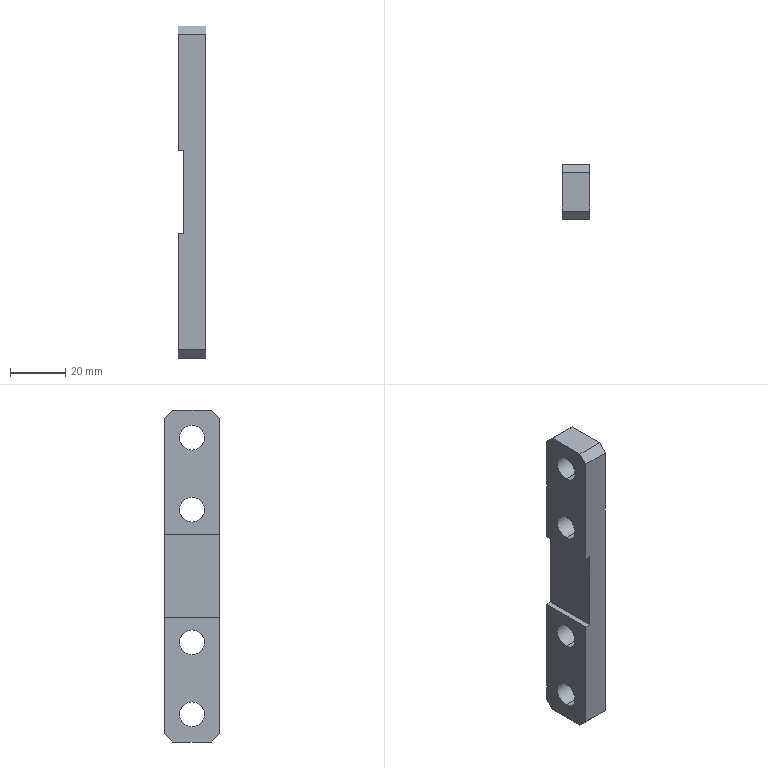Part | SolidWorks | features HoleWzd 2, Chamfer 1, Extrusion 1, ICE 1 | 1 solid | 22 faces | box 10 x 20 x 120 mm | volume 20075 mm3 | plane 14 | cylinder 8 | commonest cylinder face diameters 9 x8
STEP:
#1=CARTESIAN_POINT('',(10.,0.,-54.5));
#2=VERTEX_POINT('',#1);
#3=CARTESIAN_POINT('',(10.,0.,-45.5));
#4=VERTEX_POINT('',#3);
#5=CARTESIAN_POINT('',(10.,0.,-50.));
#6=DIRECTION('',(-1.,0.,0.));
#7=DIRECTION('',(0.,0.,1.));
#8=AXIS2_PLACEMENT_3D('',#5,#6,#7);
#9=CIRCLE('',#8,4.5);
#10=EDGE_CURVE('',#2,#4,#9,.T.);
#11=ORIENTED_EDGE('',*,*,#10,.F.);
#12=CARTESIAN_POINT('',(0.,0.,-54.5));
#13=VERTEX_POINT('',#12);
#14=CARTESIAN_POINT('',(0.,0.,-54.5));
#15=DIRECTION('',(-1.,0.,0.));
#16=VECTOR('',#15,1000.);
#17=LINE('',#14,#16);
#18=EDGE_CURVE('',#2,#13,#17,.T.);
#19=ORIENTED_EDGE('',*,*,#18,.T.);
#20=CARTESIAN_POINT('',(0.,0.,-45.5));
#21=VERTEX_POINT('',#20);
#22=CARTESIAN_POINT('',(0.,0.,-50.));
#23=DIRECTION('',(-1.,0.,0.));
#24=DIRECTION('',(0.,0.,1.));
#25=AXIS2_PLACEMENT_3D('',#22,#23,#24);
#26=CIRCLE('',#25,4.5);
#27=EDGE_CURVE('',#13,#21,#26,.T.);
#28=ORIENTED_EDGE('',*,*,#27,.T.);
#29=CARTESIAN_POINT('',(0.,0.,-45.5));
#30=DIRECTION('',(-1.,0.,0.));
#31=VECTOR('',#30,1000.);
#32=LINE('',#29,#31);
#33=EDGE_CURVE('',#4,#21,#32,.T.);
#34=ORIENTED_EDGE('',*,*,#33,.F.);
#35=EDGE_LOOP('',(#11,#19,#28,#34));
#36=FACE_OUTER_BOUND('',#35,.T.);
#37=CARTESIAN_POINT('',(0.,0.,-50.));
#38=DIRECTION('',(-1.,0.,0.));
#39=DIRECTION('',(0.,0.,1.));
#40=AXIS2_PLACEMENT_3D('',#37,#38,#39);
#41=CYLINDRICAL_SURFACE('',#40,4.5);
#42=ADVANCED_FACE('',(#36),#41,.F.);
#43=CARTESIAN_POINT('',(10.,0.,45.5));
#44=VERTEX_POINT('',#43);
#45=CARTESIAN_POINT('',(10.,0.,54.5));
#46=VERTEX_POINT('',#45);
#47=CARTESIAN_POINT('',(10.,0.,50.));
#48=DIRECTION('',(-1.,0.,0.));
#49=DIRECTION('',(0.,0.,1.));
#50=AXIS2_PLACEMENT_3D('',#47,#48,#49);
#51=CIRCLE('',#50,4.5);
#52=EDGE_CURVE('',#44,#46,#51,.T.);
#53=ORIENTED_EDGE('',*,*,#52,.F.);
#54=CARTESIAN_POINT('',(0.,0.,45.5));
#55=VERTEX_POINT('',#54);
#56=CARTESIAN_POINT('',(0.,0.,45.5));
#57=DIRECTION('',(-1.,0.,0.));
#58=VECTOR('',#57,1000.);
#59=LINE('',#56,#58);
#60=EDGE_CURVE('',#44,#55,#59,.T.);
#61=ORIENTED_EDGE('',*,*,#60,.T.);
#62=CARTESIAN_POINT('',(0.,0.,54.5));
#63=VERTEX_POINT('',#62);
#64=CARTESIAN_POINT('',(0.,0.,50.));
#65=DIRECTION('',(-1.,0.,0.));
#66=DIRECTION('',(0.,0.,1.));
#67=AXIS2_PLACEMENT_3D('',#64,#65,#66);
#68=CIRCLE('',#67,4.5);
#69=EDGE_CURVE('',#55,#63,#68,.T.);
#70=ORIENTED_EDGE('',*,*,#69,.T.);
#71=CARTESIAN_POINT('',(0.,0.,54.5));
#72=DIRECTION('',(-1.,0.,0.));
#73=VECTOR('',#72,1000.);
#74=LINE('',#71,#73);
#75=EDGE_CURVE('',#46,#63,#74,.T.);
#76=ORIENTED_EDGE('',*,*,#75,.F.);
#77=EDGE_LOOP('',(#53,#61,#70,#76));
#78=FACE_OUTER_BOUND('',#77,.T.);
#79=CARTESIAN_POINT('',(0.,0.,50.));
#80=DIRECTION('',(-1.,0.,0.));
#81=DIRECTION('',(0.,0.,1.));
#82=AXIS2_PLACEMENT_3D('',#79,#80,#81);
#83=CYLINDRICAL_SURFACE('',#82,4.5);
#84=ADVANCED_FACE('',(#78),#83,.F.);
#85=CARTESIAN_POINT('',(0.,0.,28.5));
#86=VERTEX_POINT('',#85);
#87=CARTESIAN_POINT('',(0.,0.,19.5));
#88=VERTEX_POINT('',#87);
#89=CARTESIAN_POINT('',(0.,0.,24.));
#90=DIRECTION('',(1.,0.,0.));
#91=DIRECTION('',(0.,0.,-1.));
#92=AXIS2_PLACEMENT_3D('',#89,#90,#91);
#93=CIRCLE('',#92,4.5);
#94=EDGE_CURVE('',#86,#88,#93,.T.);
#95=ORIENTED_EDGE('',*,*,#94,.F.);
#96=CARTESIAN_POINT('',(10.,0.,28.5));
#97=VERTEX_POINT('',#96);
#98=CARTESIAN_POINT('',(10.,0.,28.5));
#99=DIRECTION('',(1.,0.,0.));
#100=VECTOR('',#99,1000.);
#101=LINE('',#98,#100);
#102=EDGE_CURVE('',#86,#97,#101,.T.);
#103=ORIENTED_EDGE('',*,*,#102,.T.);
#104=CARTESIAN_POINT('',(10.,0.,19.5));
#105=VERTEX_POINT('',#104);
#106=CARTESIAN_POINT('',(10.,0.,24.));
#107=DIRECTION('',(1.,0.,0.));
#108=DIRECTION('',(0.,0.,-1.));
#109=AXIS2_PLACEMENT_3D('',#106,#107,#108);
#110=CIRCLE('',#109,4.5);
#111=EDGE_CURVE('',#97,#105,#110,.T.);
#112=ORIENTED_EDGE('',*,*,#111,.T.);
#113=CARTESIAN_POINT('',(10.,0.,19.5));
#114=DIRECTION('',(1.,0.,0.));
#115=VECTOR('',#114,1000.);
#116=LINE('',#113,#115);
#117=EDGE_CURVE('',#88,#105,#116,.T.);
#118=ORIENTED_EDGE('',*,*,#117,.F.);
#119=EDGE_LOOP('',(#95,#103,#112,#118));
#120=FACE_OUTER_BOUND('',#119,.T.);
#121=CARTESIAN_POINT('',(10.,0.,24.));
#122=DIRECTION('',(1.,0.,0.));
#123=DIRECTION('',(0.,0.,-1.));
#124=AXIS2_PLACEMENT_3D('',#121,#122,#123);
#125=CYLINDRICAL_SURFACE('',#124,4.5);
#126=ADVANCED_FACE('',(#120),#125,.F.);
#127=CARTESIAN_POINT('',(0.,0.,-19.5));
#128=VERTEX_POINT('',#127);
#129=CARTESIAN_POINT('',(0.,0.,-28.5));
#130=VERTEX_POINT('',#129);
#131=CARTESIAN_POINT('',(0.,0.,-24.));
#132=DIRECTION('',(1.,0.,0.));
#133=DIRECTION('',(0.,0.,-1.));
#134=AXIS2_PLACEMENT_3D('',#131,#132,#133);
#135=CIRCLE('',#134,4.5);
#136=EDGE_CURVE('',#128,#130,#135,.T.);
#137=ORIENTED_EDGE('',*,*,#136,.F.);
#138=CARTESIAN_POINT('',(10.,0.,-19.5));
#139=VERTEX_POINT('',#138);
#140=CARTESIAN_POINT('',(10.,0.,-19.5));
#141=DIRECTION('',(1.,0.,0.));
#142=VECTOR('',#141,1000.);
#143=LINE('',#140,#142);
#144=EDGE_CURVE('',#128,#139,#143,.T.);
#145=ORIENTED_EDGE('',*,*,#144,.T.);
#146=CARTESIAN_POINT('',(10.,0.,-28.5));
#147=VERTEX_POINT('',#146);
#148=CARTESIAN_POINT('',(10.,0.,-24.));
#149=DIRECTION('',(1.,0.,0.));
#150=DIRECTION('',(0.,0.,-1.));
#151=AXIS2_PLACEMENT_3D('',#148,#149,#150);
#152=CIRCLE('',#151,4.5);
#153=EDGE_CURVE('',#139,#147,#152,.T.);
#154=ORIENTED_EDGE('',*,*,#153,.T.);
#155=CARTESIAN_POINT('',(10.,0.,-28.5));
#156=DIRECTION('',(1.,0.,0.));
#157=VECTOR('',#156,1000.);
#158=LINE('',#155,#157);
#159=EDGE_CURVE('',#130,#147,#158,.T.);
#160=ORIENTED_EDGE('',*,*,#159,.F.);
#161=EDGE_LOOP('',(#137,#145,#154,#160));
#162=FACE_OUTER_BOUND('',#161,.T.);
#163=CARTESIAN_POINT('',(10.,0.,-24.));
#164=DIRECTION('',(1.,0.,0.));
#165=DIRECTION('',(0.,0.,-1.));
#166=AXIS2_PLACEMENT_3D('',#163,#164,#165);
#167=CYLINDRICAL_SURFACE('',#166,4.5);
#168=ADVANCED_FACE('',(#162),#167,.F.);
#169=CARTESIAN_POINT('',(10.,10.,-57.));
#170=VERTEX_POINT('',#169);
#171=CARTESIAN_POINT('',(10.,10.,57.));
#172=VERTEX_POINT('',#171);
#173=CARTESIAN_POINT('',(10.,10.,60.));
#174=DIRECTION('',(0.,0.,1.));
#175=VECTOR('',#174,1000.);
#176=LINE('',#173,#175);
#177=EDGE_CURVE('',#170,#172,#176,.T.);
#178=ORIENTED_EDGE('',*,*,#177,.F.);
#179=CARTESIAN_POINT('',(0.,10.,-57.));
#180=VERTEX_POINT('',#179);
#181=CARTESIAN_POINT('',(10.,10.,-57.));
#182=DIRECTION('',(-1.,0.,0.));
#183=VECTOR('',#182,1000.);
#184=LINE('',#181,#183);
#185=EDGE_CURVE('',#170,#180,#184,.T.);
#186=ORIENTED_EDGE('',*,*,#185,.T.);
#187=CARTESIAN_POINT('',(0.,10.,-15.));
#188=VERTEX_POINT('',#187);
#189=CARTESIAN_POINT('',(0.,10.,60.));
#190=DIRECTION('',(0.,0.,1.));
#191=VECTOR('',#190,1000.);
#192=LINE('',#189,#191);
#193=EDGE_CURVE('',#180,#188,#192,.T.);
#194=ORIENTED_EDGE('',*,*,#193,.T.);
#195=CARTESIAN_POINT('',(2.,10.,-15.));
#196=VERTEX_POINT('',#195);
#197=CARTESIAN_POINT('',(2.,10.,-15.));
#198=DIRECTION('',(-1.,0.,0.));
#199=VECTOR('',#198,1000.);
#200=LINE('',#197,#199);
#201=EDGE_CURVE('',#196,#188,#200,.T.);
#202=ORIENTED_EDGE('',*,*,#201,.F.);
#203=CARTESIAN_POINT('',(2.,10.,15.));
#204=VERTEX_POINT('',#203);
#205=CARTESIAN_POINT('',(2.,10.,15.));
#206=DIRECTION('',(0.,0.,1.));
#207=VECTOR('',#206,1000.);
#208=LINE('',#205,#207);
#209=EDGE_CURVE('',#196,#204,#208,.T.);
#210=ORIENTED_EDGE('',*,*,#209,.T.);
#211=CARTESIAN_POINT('',(0.,10.,15.));
#212=VERTEX_POINT('',#211);
#213=CARTESIAN_POINT('',(2.,10.,15.));
#214=DIRECTION('',(-1.,0.,0.));
#215=VECTOR('',#214,1000.);
#216=LINE('',#213,#215);
#217=EDGE_CURVE('',#204,#212,#216,.T.);
#218=ORIENTED_EDGE('',*,*,#217,.T.);
#219=CARTESIAN_POINT('',(0.,10.,57.));
#220=VERTEX_POINT('',#219);
#221=CARTESIAN_POINT('',(0.,10.,60.));
#222=DIRECTION('',(0.,0.,1.));
#223=VECTOR('',#222,1000.);
#224=LINE('',#221,#223);
#225=EDGE_CURVE('',#212,#220,#224,.T.);
#226=ORIENTED_EDGE('',*,*,#225,.T.);
#227=CARTESIAN_POINT('',(10.,10.,57.));
#228=DIRECTION('',(1.,0.,0.));
#229=VECTOR('',#228,1000.);
#230=LINE('',#227,#229);
#231=EDGE_CURVE('',#220,#172,#230,.T.);
#232=ORIENTED_EDGE('',*,*,#231,.T.);
#233=EDGE_LOOP('',(#178,#186,#194,#202,#210,#218,#226,#232));
#234=FACE_OUTER_BOUND('',#233,.T.);
#235=CARTESIAN_POINT('',(10.,10.,60.));
#236=DIRECTION('',(0.,-1.,0.));
#237=DIRECTION('',(0.,0.,-1.));
#238=AXIS2_PLACEMENT_3D('',#235,#236,#237);
#239=PLANE('',#238);
#240=ADVANCED_FACE('',(#234),#239,.F.);
#241=CARTESIAN_POINT('',(0.,-10.,-15.));
#242=VERTEX_POINT('',#241);
#243=CARTESIAN_POINT('',(0.,-10.,-57.));
#244=VERTEX_POINT('',#243);
#245=CARTESIAN_POINT('',(0.,-10.,60.));
#246=DIRECTION('',(0.,0.,-1.));
#247=VECTOR('',#246,1000.);
#248=LINE('',#245,#247);
#249=EDGE_CURVE('',#242,#244,#248,.T.);
#250=ORIENTED_EDGE('',*,*,#249,.T.);
#251=CARTESIAN_POINT('',(10.,-10.,-57.));
#252=VERTEX_POINT('',#251);
#253=CARTESIAN_POINT('',(10.,-10.,-57.));
#254=DIRECTION('',(1.,0.,0.));
#255=VECTOR('',#254,1000.);
#256=LINE('',#253,#255);
#257=EDGE_CURVE('',#244,#252,#256,.T.);
#258=ORIENTED_EDGE('',*,*,#257,.T.);
#259=CARTESIAN_POINT('',(10.,-10.,57.));
#260=VERTEX_POINT('',#259);
#261=CARTESIAN_POINT('',(10.,-10.,60.));
#262=DIRECTION('',(0.,0.,-1.));
#263=VECTOR('',#262,1000.);
#264=LINE('',#261,#263);
#265=EDGE_CURVE('',#260,#252,#264,.T.);
#266=ORIENTED_EDGE('',*,*,#265,.F.);
#267=CARTESIAN_POINT('',(0.,-10.,57.));
#268=VERTEX_POINT('',#267);
#269=CARTESIAN_POINT('',(10.,-10.,57.));
#270=DIRECTION('',(-1.,0.,0.));
#271=VECTOR('',#270,1000.);
#272=LINE('',#269,#271);
#273=EDGE_CURVE('',#260,#268,#272,.T.);
#274=ORIENTED_EDGE('',*,*,#273,.T.);
#275=CARTESIAN_POINT('',(0.,-10.,15.));
#276=VERTEX_POINT('',#275);
#277=CARTESIAN_POINT('',(0.,-10.,60.));
#278=DIRECTION('',(0.,0.,-1.));
#279=VECTOR('',#278,1000.);
#280=LINE('',#277,#279);
#281=EDGE_CURVE('',#268,#276,#280,.T.);
#282=ORIENTED_EDGE('',*,*,#281,.T.);
#283=CARTESIAN_POINT('',(2.,-10.,15.));
#284=VERTEX_POINT('',#283);
#285=CARTESIAN_POINT('',(2.,-10.,15.));
#286=DIRECTION('',(-1.,0.,0.));
#287=VECTOR('',#286,1000.);
#288=LINE('',#285,#287);
#289=EDGE_CURVE('',#284,#276,#288,.T.);
#290=ORIENTED_EDGE('',*,*,#289,.F.);
#291=CARTESIAN_POINT('',(2.,-10.,-15.));
#292=VERTEX_POINT('',#291);
#293=CARTESIAN_POINT('',(2.,-10.,15.));
#294=DIRECTION('',(0.,0.,-1.));
#295=VECTOR('',#294,1000.);
#296=LINE('',#293,#295);
#297=EDGE_CURVE('',#284,#292,#296,.T.);
#298=ORIENTED_EDGE('',*,*,#297,.T.);
#299=CARTESIAN_POINT('',(2.,-10.,-15.));
#300=DIRECTION('',(-1.,0.,0.));
#301=VECTOR('',#300,1000.);
#302=LINE('',#299,#301);
#303=EDGE_CURVE('',#292,#242,#302,.T.);
#304=ORIENTED_EDGE('',*,*,#303,.T.);
#305=EDGE_LOOP('',(#250,#258,#266,#274,#282,#290,#298,#304));
#306=FACE_OUTER_BOUND('',#305,.T.);
#307=CARTESIAN_POINT('',(10.,-10.,60.));
#308=DIRECTION('',(0.,1.,0.));
#309=DIRECTION('',(0.,0.,1.));
#310=AXIS2_PLACEMENT_3D('',#307,#308,#309);
#311=PLANE('',#310);
#312=ADVANCED_FACE('',(#306),#311,.F.);
#313=CARTESIAN_POINT('',(0.,0.,-24.));
#314=DIRECTION('',(1.,0.,0.));
#315=DIRECTION('',(0.,0.,-1.));
#316=AXIS2_PLACEMENT_3D('',#313,#314,#315);
#317=CIRCLE('',#316,4.5);
#318=EDGE_CURVE('',#130,#128,#317,.T.);
#319=ORIENTED_EDGE('',*,*,#318,.T.);
#320=ORIENTED_EDGE('',*,*,#136,.T.);
#321=EDGE_LOOP('',(#319,#320));
#322=FACE_BOUND('',#321,.T.);
#323=CARTESIAN_POINT('',(0.,0.,-50.));
#324=DIRECTION('',(-1.,0.,0.));
#325=DIRECTION('',(0.,0.,1.));
#326=AXIS2_PLACEMENT_3D('',#323,#324,#325);
#327=CIRCLE('',#326,4.5);
#328=EDGE_CURVE('',#21,#13,#327,.T.);
#329=ORIENTED_EDGE('',*,*,#328,.F.);
#330=ORIENTED_EDGE('',*,*,#27,.F.);
#331=EDGE_LOOP('',(#329,#330));
#332=FACE_BOUND('',#331,.T.);
#333=CARTESIAN_POINT('',(0.,-7.,-60.));
#334=VERTEX_POINT('',#333);
#335=CARTESIAN_POINT('',(0.,7.,-60.));
#336=VERTEX_POINT('',#335);
#337=CARTESIAN_POINT('',(0.,10.,-60.));
#338=DIRECTION('',(0.,1.,0.));
#339=VECTOR('',#338,1000.);
#340=LINE('',#337,#339);
#341=EDGE_CURVE('',#334,#336,#340,.T.);
#342=ORIENTED_EDGE('',*,*,#341,.F.);
#343=CARTESIAN_POINT('',(0.,-7.,-60.));
#344=DIRECTION('',(0.,-0.7071,0.7071));
#345=VECTOR('',#344,1000.);
#346=LINE('',#343,#345);
#347=EDGE_CURVE('',#334,#244,#346,.T.);
#348=ORIENTED_EDGE('',*,*,#347,.T.);
#349=ORIENTED_EDGE('',*,*,#249,.F.);
#350=CARTESIAN_POINT('',(0.,10.,-15.));
#351=DIRECTION('',(0.,1.,0.));
#352=VECTOR('',#351,1000.);
#353=LINE('',#350,#352);
#354=EDGE_CURVE('',#242,#188,#353,.T.);
#355=ORIENTED_EDGE('',*,*,#354,.T.);
#356=ORIENTED_EDGE('',*,*,#193,.F.);
#357=CARTESIAN_POINT('',(0.,10.,-57.));
#358=DIRECTION('',(0.,-0.7071,-0.7071));
#359=VECTOR('',#358,1000.);
#360=LINE('',#357,#359);
#361=EDGE_CURVE('',#180,#336,#360,.T.);
#362=ORIENTED_EDGE('',*,*,#361,.T.);
#363=EDGE_LOOP('',(#342,#348,#349,#355,#356,#362));
#364=FACE_OUTER_BOUND('',#363,.T.);
#365=CARTESIAN_POINT('',(0.,0.,0.));
#366=DIRECTION('',(1.,0.,0.));
#367=DIRECTION('',(0.,0.,-1.));
#368=AXIS2_PLACEMENT_3D('',#365,#366,#367);
#369=PLANE('',#368);
#370=ADVANCED_FACE('',(#322,#332,#364),#369,.F.);
#371=CARTESIAN_POINT('',(0.,0.,24.));
#372=DIRECTION('',(1.,0.,0.));
#373=DIRECTION('',(0.,0.,-1.));
#374=AXIS2_PLACEMENT_3D('',#371,#372,#373);
#375=CIRCLE('',#374,4.5);
#376=EDGE_CURVE('',#88,#86,#375,.T.);
#377=ORIENTED_EDGE('',*,*,#376,.T.);
#378=ORIENTED_EDGE('',*,*,#94,.T.);
#379=EDGE_LOOP('',(#377,#378));
#380=FACE_BOUND('',#379,.T.);
#381=CARTESIAN_POINT('',(0.,0.,50.));
#382=DIRECTION('',(-1.,0.,0.));
#383=DIRECTION('',(0.,0.,1.));
#384=AXIS2_PLACEMENT_3D('',#381,#382,#383);
#385=CIRCLE('',#384,4.5);
#386=EDGE_CURVE('',#63,#55,#385,.T.);
#387=ORIENTED_EDGE('',*,*,#386,.F.);
#388=ORIENTED_EDGE('',*,*,#69,.F.);
#389=EDGE_LOOP('',(#387,#388));
#390=FACE_BOUND('',#389,.T.);
#391=ORIENTED_EDGE('',*,*,#281,.F.);
#392=CARTESIAN_POINT('',(0.,-7.,60.));
#393=VERTEX_POINT('',#392);
#394=CARTESIAN_POINT('',(0.,-10.,57.));
#395=DIRECTION('',(0.,0.7071,0.7071));
#396=VECTOR('',#395,1000.);
#397=LINE('',#394,#396);
#398=EDGE_CURVE('',#268,#393,#397,.T.);
#399=ORIENTED_EDGE('',*,*,#398,.T.);
#400=CARTESIAN_POINT('',(0.,7.,60.));
#401=VERTEX_POINT('',#400);
#402=CARTESIAN_POINT('',(0.,10.,60.));
#403=DIRECTION('',(0.,-1.,0.));
#404=VECTOR('',#403,1000.);
#405=LINE('',#402,#404);
#406=EDGE_CURVE('',#401,#393,#405,.T.);
#407=ORIENTED_EDGE('',*,*,#406,.F.);
#408=CARTESIAN_POINT('',(0.,7.,60.));
#409=DIRECTION('',(0.,0.7071,-0.7071));
#410=VECTOR('',#409,1000.);
#411=LINE('',#408,#410);
#412=EDGE_CURVE('',#401,#220,#411,.T.);
#413=ORIENTED_EDGE('',*,*,#412,.T.);
#414=ORIENTED_EDGE('',*,*,#225,.F.);
#415=CARTESIAN_POINT('',(0.,10.,15.));
#416=DIRECTION('',(0.,-1.,0.));
#417=VECTOR('',#416,1000.);
#418=LINE('',#415,#417);
#419=EDGE_CURVE('',#212,#276,#418,.T.);
#420=ORIENTED_EDGE('',*,*,#419,.T.);
#421=EDGE_LOOP('',(#391,#399,#407,#413,#414,#420));
#422=FACE_OUTER_BOUND('',#421,.T.);
#423=CARTESIAN_POINT('',(0.,0.,0.));
#424=DIRECTION('',(1.,0.,0.));
#425=DIRECTION('',(0.,0.,-1.));
#426=AXIS2_PLACEMENT_3D('',#423,#424,#425);
#427=PLANE('',#426);
#428=ADVANCED_FACE('',(#380,#390,#422),#427,.F.);
#429=CARTESIAN_POINT('',(10.,-7.,-60.));
#430=VERTEX_POINT('',#429);
#431=CARTESIAN_POINT('',(10.,7.,-60.));
#432=VERTEX_POINT('',#431);
#433=CARTESIAN_POINT('',(10.,10.,-60.));
#434=DIRECTION('',(0.,1.,0.));
#435=VECTOR('',#434,1000.);
#436=LINE('',#433,#435);
#437=EDGE_CURVE('',#430,#432,#436,.T.);
#438=ORIENTED_EDGE('',*,*,#437,.F.);
#439=CARTESIAN_POINT('',(10.,-7.,-60.));
#440=DIRECTION('',(-1.,0.,0.));
#441=VECTOR('',#440,1000.);
#442=LINE('',#439,#441);
#443=EDGE_CURVE('',#430,#334,#442,.T.);
#444=ORIENTED_EDGE('',*,*,#443,.T.);
#445=ORIENTED_EDGE('',*,*,#341,.T.);
#446=CARTESIAN_POINT('',(10.,7.,-60.));
#447=DIRECTION('',(1.,0.,0.));
#448=VECTOR('',#447,1000.);
#449=LINE('',#446,#448);
#450=EDGE_CURVE('',#336,#432,#449,.T.);
#451=ORIENTED_EDGE('',*,*,#450,.T.);
#452=EDGE_LOOP('',(#438,#444,#445,#451));
#453=FACE_OUTER_BOUND('',#452,.T.);
#454=CARTESIAN_POINT('',(10.,10.,-60.));
#455=DIRECTION('',(0.,0.,1.));
#456=DIRECTION('',(1.,0.,0.));
#457=AXIS2_PLACEMENT_3D('',#454,#455,#456);
#458=PLANE('',#457);
#459=ADVANCED_FACE('',(#453),#458,.F.);
#460=ORIENTED_EDGE('',*,*,#406,.T.);
#461=CARTESIAN_POINT('',(10.,-7.,60.));
#462=VERTEX_POINT('',#461);
#463=CARTESIAN_POINT('',(10.,-7.,60.));
#464=DIRECTION('',(1.,0.,0.));
#465=VECTOR('',#464,1000.);
#466=LINE('',#463,#465);
#467=EDGE_CURVE('',#393,#462,#466,.T.);
#468=ORIENTED_EDGE('',*,*,#467,.T.);
#469=CARTESIAN_POINT('',(10.,7.,60.));
#470=VERTEX_POINT('',#469);
#471=CARTESIAN_POINT('',(10.,10.,60.));
#472=DIRECTION('',(0.,-1.,0.));
#473=VECTOR('',#472,1000.);
#474=LINE('',#471,#473);
#475=EDGE_CURVE('',#470,#462,#474,.T.);
#476=ORIENTED_EDGE('',*,*,#475,.F.);
#477=CARTESIAN_POINT('',(10.,7.,60.));
#478=DIRECTION('',(-1.,0.,0.));
#479=VECTOR('',#478,1000.);
#480=LINE('',#477,#479);
#481=EDGE_CURVE('',#470,#401,#480,.T.);
#482=ORIENTED_EDGE('',*,*,#481,.T.);
#483=EDGE_LOOP('',(#460,#468,#476,#482));
#484=FACE_OUTER_BOUND('',#483,.T.);
#485=CARTESIAN_POINT('',(10.,10.,60.));
#486=DIRECTION('',(0.,0.,-1.));
#487=DIRECTION('',(-1.,0.,0.));
#488=AXIS2_PLACEMENT_3D('',#485,#486,#487);
#489=PLANE('',#488);
#490=ADVANCED_FACE('',(#484),#489,.F.);
#491=CARTESIAN_POINT('',(10.,0.,-50.));
#492=DIRECTION('',(-1.,0.,0.));
#493=DIRECTION('',(0.,0.,1.));
#494=AXIS2_PLACEMENT_3D('',#491,#492,#493);
#495=CIRCLE('',#494,4.5);
#496=EDGE_CURVE('',#4,#2,#495,.T.);
#497=ORIENTED_EDGE('',*,*,#496,.T.);
#498=ORIENTED_EDGE('',*,*,#10,.T.);
#499=EDGE_LOOP('',(#497,#498));
#500=FACE_BOUND('',#499,.T.);
#501=CARTESIAN_POINT('',(10.,0.,50.));
#502=DIRECTION('',(-1.,0.,0.));
#503=DIRECTION('',(0.,0.,1.));
#504=AXIS2_PLACEMENT_3D('',#501,#502,#503);
#505=CIRCLE('',#504,4.5);
#506=EDGE_CURVE('',#46,#44,#505,.T.);
#507=ORIENTED_EDGE('',*,*,#506,.T.);
#508=ORIENTED_EDGE('',*,*,#52,.T.);
#509=EDGE_LOOP('',(#507,#508));
#510=FACE_BOUND('',#509,.T.);
#511=CARTESIAN_POINT('',(10.,0.,24.));
#512=DIRECTION('',(1.,0.,0.));
#513=DIRECTION('',(0.,0.,-1.));
#514=AXIS2_PLACEMENT_3D('',#511,#512,#513);
#515=CIRCLE('',#514,4.5);
#516=EDGE_CURVE('',#105,#97,#515,.T.);
#517=ORIENTED_EDGE('',*,*,#516,.F.);
#518=ORIENTED_EDGE('',*,*,#111,.F.);
#519=EDGE_LOOP('',(#517,#518));
#520=FACE_BOUND('',#519,.T.);
#521=CARTESIAN_POINT('',(10.,0.,-24.));
#522=DIRECTION('',(1.,0.,0.));
#523=DIRECTION('',(0.,0.,-1.));
#524=AXIS2_PLACEMENT_3D('',#521,#522,#523);
#525=CIRCLE('',#524,4.5);
#526=EDGE_CURVE('',#147,#139,#525,.T.);
#527=ORIENTED_EDGE('',*,*,#526,.F.);
#528=ORIENTED_EDGE('',*,*,#153,.F.);
#529=EDGE_LOOP('',(#527,#528));
#530=FACE_BOUND('',#529,.T.);
#531=ORIENTED_EDGE('',*,*,#265,.T.);
#532=CARTESIAN_POINT('',(10.,-33.5,-33.5));
#533=DIRECTION('',(0.,0.7071,-0.7071));
#534=VECTOR('',#533,1000.);
#535=LINE('',#532,#534);
#536=EDGE_CURVE('',#252,#430,#535,.T.);
#537=ORIENTED_EDGE('',*,*,#536,.T.);
#538=ORIENTED_EDGE('',*,*,#437,.T.);
#539=CARTESIAN_POINT('',(10.,33.5,-33.5));
#540=DIRECTION('',(0.,0.7071,0.7071));
#541=VECTOR('',#540,1000.);
#542=LINE('',#539,#541);
#543=EDGE_CURVE('',#432,#170,#542,.T.);
#544=ORIENTED_EDGE('',*,*,#543,.T.);
#545=ORIENTED_EDGE('',*,*,#177,.T.);
#546=CARTESIAN_POINT('',(10.,33.5,33.5));
#547=DIRECTION('',(0.,-0.7071,0.7071));
#548=VECTOR('',#547,1000.);
#549=LINE('',#546,#548);
#550=EDGE_CURVE('',#172,#470,#549,.T.);
#551=ORIENTED_EDGE('',*,*,#550,.T.);
#552=ORIENTED_EDGE('',*,*,#475,.T.);
#553=CARTESIAN_POINT('',(10.,-33.5,33.5));
#554=DIRECTION('',(0.,-0.7071,-0.7071));
#555=VECTOR('',#554,1000.);
#556=LINE('',#553,#555);
#557=EDGE_CURVE('',#462,#260,#556,.T.);
#558=ORIENTED_EDGE('',*,*,#557,.T.);
#559=EDGE_LOOP('',(#531,#537,#538,#544,#545,#551,#552,#558));
#560=FACE_OUTER_BOUND('',#559,.T.);
#561=CARTESIAN_POINT('',(10.,0.,0.));
#562=DIRECTION('',(1.,0.,0.));
#563=DIRECTION('',(0.,0.,-1.));
#564=AXIS2_PLACEMENT_3D('',#561,#562,#563);
#565=PLANE('',#564);
#566=ADVANCED_FACE('',(#500,#510,#520,#530,#560),#565,.T.);
#567=ORIENTED_EDGE('',*,*,#144,.F.);
#568=ORIENTED_EDGE('',*,*,#318,.F.);
#569=ORIENTED_EDGE('',*,*,#159,.T.);
#570=ORIENTED_EDGE('',*,*,#526,.T.);
#571=EDGE_LOOP('',(#567,#568,#569,#570));
#572=FACE_OUTER_BOUND('',#571,.T.);
#573=CARTESIAN_POINT('',(10.,0.,-24.));
#574=DIRECTION('',(1.,0.,0.));
#575=DIRECTION('',(0.,0.,-1.));
#576=AXIS2_PLACEMENT_3D('',#573,#574,#575);
#577=CYLINDRICAL_SURFACE('',#576,4.5);
#578=ADVANCED_FACE('',(#572),#577,.F.);
#579=ORIENTED_EDGE('',*,*,#102,.F.);
#580=ORIENTED_EDGE('',*,*,#376,.F.);
#581=ORIENTED_EDGE('',*,*,#117,.T.);
#582=ORIENTED_EDGE('',*,*,#516,.T.);
#583=EDGE_LOOP('',(#579,#580,#581,#582));
#584=FACE_OUTER_BOUND('',#583,.T.);
#585=CARTESIAN_POINT('',(10.,0.,24.));
#586=DIRECTION('',(1.,0.,0.));
#587=DIRECTION('',(0.,0.,-1.));
#588=AXIS2_PLACEMENT_3D('',#585,#586,#587);
#589=CYLINDRICAL_SURFACE('',#588,4.5);
#590=ADVANCED_FACE('',(#584),#589,.F.);
#591=ORIENTED_EDGE('',*,*,#60,.F.);
#592=ORIENTED_EDGE('',*,*,#506,.F.);
#593=ORIENTED_EDGE('',*,*,#75,.T.);
#594=ORIENTED_EDGE('',*,*,#386,.T.);
#595=EDGE_LOOP('',(#591,#592,#593,#594));
#596=FACE_OUTER_BOUND('',#595,.T.);
#597=CARTESIAN_POINT('',(0.,0.,50.));
#598=DIRECTION('',(-1.,0.,0.));
#599=DIRECTION('',(0.,0.,1.));
#600=AXIS2_PLACEMENT_3D('',#597,#598,#599);
#601=CYLINDRICAL_SURFACE('',#600,4.5);
#602=ADVANCED_FACE('',(#596),#601,.F.);
#603=ORIENTED_EDGE('',*,*,#18,.F.);
#604=ORIENTED_EDGE('',*,*,#496,.F.);
#605=ORIENTED_EDGE('',*,*,#33,.T.);
#606=ORIENTED_EDGE('',*,*,#328,.T.);
#607=EDGE_LOOP('',(#603,#604,#605,#606));
#608=FACE_OUTER_BOUND('',#607,.T.);
#609=CARTESIAN_POINT('',(0.,0.,-50.));
#610=DIRECTION('',(-1.,0.,0.));
#611=DIRECTION('',(0.,0.,1.));
#612=AXIS2_PLACEMENT_3D('',#609,#610,#611);
#613=CYLINDRICAL_SURFACE('',#612,4.5);
#614=ADVANCED_FACE('',(#608),#613,.F.);
#615=ORIENTED_EDGE('',*,*,#354,.F.);
#616=ORIENTED_EDGE('',*,*,#303,.F.);
#617=CARTESIAN_POINT('',(2.,10.,-15.));
#618=DIRECTION('',(0.,1.,0.));
#619=VECTOR('',#618,1000.);
#620=LINE('',#617,#619);
#621=EDGE_CURVE('',#292,#196,#620,.T.);
#622=ORIENTED_EDGE('',*,*,#621,.T.);
#623=ORIENTED_EDGE('',*,*,#201,.T.);
#624=EDGE_LOOP('',(#615,#616,#622,#623));
#625=FACE_OUTER_BOUND('',#624,.T.);
#626=CARTESIAN_POINT('',(2.,10.,-15.));
#627=DIRECTION('',(0.,0.,1.));
#628=DIRECTION('',(1.,0.,0.));
#629=AXIS2_PLACEMENT_3D('',#626,#627,#628);
#630=PLANE('',#629);
#631=ADVANCED_FACE('',(#625),#630,.T.);
#632=ORIENTED_EDGE('',*,*,#419,.F.);
#633=ORIENTED_EDGE('',*,*,#217,.F.);
#634=CARTESIAN_POINT('',(2.,10.,15.));
#635=DIRECTION('',(0.,-1.,0.));
#636=VECTOR('',#635,1000.);
#637=LINE('',#634,#636);
#638=EDGE_CURVE('',#204,#284,#637,.T.);
#639=ORIENTED_EDGE('',*,*,#638,.T.);
#640=ORIENTED_EDGE('',*,*,#289,.T.);
#641=EDGE_LOOP('',(#632,#633,#639,#640));
#642=FACE_OUTER_BOUND('',#641,.T.);
#643=CARTESIAN_POINT('',(2.,10.,15.));
#644=DIRECTION('',(0.,0.,-1.));
#645=DIRECTION('',(-1.,0.,0.));
#646=AXIS2_PLACEMENT_3D('',#643,#644,#645);
#647=PLANE('',#646);
#648=ADVANCED_FACE('',(#642),#647,.T.);
#649=ORIENTED_EDGE('',*,*,#621,.F.);
#650=ORIENTED_EDGE('',*,*,#297,.F.);
#651=ORIENTED_EDGE('',*,*,#638,.F.);
#652=ORIENTED_EDGE('',*,*,#209,.F.);
#653=EDGE_LOOP('',(#649,#650,#651,#652));
#654=FACE_OUTER_BOUND('',#653,.T.);
#655=CARTESIAN_POINT('',(2.,0.,0.));
#656=DIRECTION('',(1.,0.,0.));
#657=DIRECTION('',(0.,0.,-1.));
#658=AXIS2_PLACEMENT_3D('',#655,#656,#657);
#659=PLANE('',#658);
#660=ADVANCED_FACE('',(#654),#659,.F.);
#661=ORIENTED_EDGE('',*,*,#536,.F.);
#662=ORIENTED_EDGE('',*,*,#257,.F.);
#663=ORIENTED_EDGE('',*,*,#347,.F.);
#664=ORIENTED_EDGE('',*,*,#443,.F.);
#665=EDGE_LOOP('',(#661,#662,#663,#664));
#666=FACE_OUTER_BOUND('',#665,.T.);
#667=CARTESIAN_POINT('',(10.,-7.,-60.));
#668=DIRECTION('',(0.,0.7071,0.7071));
#669=DIRECTION('',(-1.,0.,0.));
#670=AXIS2_PLACEMENT_3D('',#667,#668,#669);
#671=PLANE('',#670);
#672=ADVANCED_FACE('',(#666),#671,.F.);
#673=ORIENTED_EDGE('',*,*,#543,.F.);
#674=ORIENTED_EDGE('',*,*,#450,.F.);
#675=ORIENTED_EDGE('',*,*,#361,.F.);
#676=ORIENTED_EDGE('',*,*,#185,.F.);
#677=EDGE_LOOP('',(#673,#674,#675,#676));
#678=FACE_OUTER_BOUND('',#677,.T.);
#679=CARTESIAN_POINT('',(10.,10.,-57.));
#680=DIRECTION('',(0.,-0.7071,0.7071));
#681=DIRECTION('',(-1.,0.,0.));
#682=AXIS2_PLACEMENT_3D('',#679,#680,#681);
#683=PLANE('',#682);
#684=ADVANCED_FACE('',(#678),#683,.F.);
#685=ORIENTED_EDGE('',*,*,#557,.F.);
#686=ORIENTED_EDGE('',*,*,#467,.F.);
#687=ORIENTED_EDGE('',*,*,#398,.F.);
#688=ORIENTED_EDGE('',*,*,#273,.F.);
#689=EDGE_LOOP('',(#685,#686,#687,#688));
#690=FACE_OUTER_BOUND('',#689,.T.);
#691=CARTESIAN_POINT('',(10.,-10.,57.));
#692=DIRECTION('',(0.,0.7071,-0.7071));
#693=DIRECTION('',(-1.,0.,0.));
#694=AXIS2_PLACEMENT_3D('',#691,#692,#693);
#695=PLANE('',#694);
#696=ADVANCED_FACE('',(#690),#695,.F.);
#697=ORIENTED_EDGE('',*,*,#550,.F.);
#698=ORIENTED_EDGE('',*,*,#231,.F.);
#699=ORIENTED_EDGE('',*,*,#412,.F.);
#700=ORIENTED_EDGE('',*,*,#481,.F.);
#701=EDGE_LOOP('',(#697,#698,#699,#700));
#702=FACE_OUTER_BOUND('',#701,.T.);
#703=CARTESIAN_POINT('',(10.,7.,60.));
#704=DIRECTION('',(0.,-0.7071,-0.7071));
#705=DIRECTION('',(-1.,0.,0.));
#706=AXIS2_PLACEMENT_3D('',#703,#704,#705);
#707=PLANE('',#706);
#708=ADVANCED_FACE('',(#702),#707,.F.);
#709=CLOSED_SHELL('',(#42,#84,#126,#168,#240,#312,#370,#428,#459,#490,#566,#578,#590,#602,#614,#631,#648,#660,#672,#684,#696,#708));
#710=MANIFOLD_SOLID_BREP('',#709);
#711=CARTESIAN_POINT('',(0.,0.,0.));
#712=DIRECTION('',(0.,0.,1.));
#713=DIRECTION('',(1.,0.,0.));
#714=AXIS2_PLACEMENT_3D('',#711,#712,#713);
#715=(LENGTH_UNIT()NAMED_UNIT(*)SI_UNIT(.MILLI.,.METRE.));
#716=UNCERTAINTY_MEASURE_WITH_UNIT(LENGTH_MEASURE(0.00001),#715,'','');
#717=(NAMED_UNIT(*)PLANE_ANGLE_UNIT()SI_UNIT($,.RADIAN.));
#718=(NAMED_UNIT(*)SI_UNIT($,.STERADIAN.)SOLID_ANGLE_UNIT());
#719=(GEOMETRIC_REPRESENTATION_CONTEXT(3)GLOBAL_UNCERTAINTY_ASSIGNED_CONTEXT((#716))GLOBAL_UNIT_ASSIGNED_CONTEXT((#715,#717,#718))REPRESENTATION_CONTEXT('',''));
#720=ADVANCED_BREP_SHAPE_REPRESENTATION('',(#710,#714),#719);